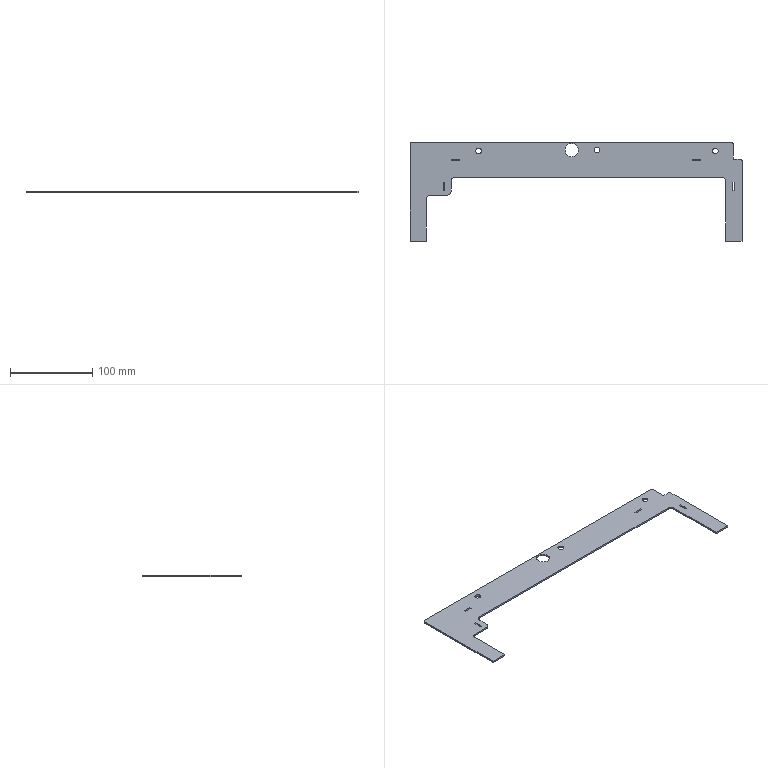Part | STEP file | xzz-001-2 | 1 solid | 45 faces | box 404 x 120 x 2 mm | volume 40299 mm3 | plane 30 | cylinder 15 | commonest cylinder face diameters 7 x6 10 x4 4 x3 16 x2
STEP:
#1=CARTESIAN_POINT('',(-138.,42.,-2.));
#2=VERTEX_POINT('',#1);
#3=CARTESIAN_POINT('',(-145.,42.,-2.));
#4=VERTEX_POINT('',#3);
#5=CARTESIAN_POINT('',(-141.5,42.,-2.));
#6=DIRECTION('',(0.,0.,-1.));
#7=DIRECTION('',(1.,0.,0.));
#8=AXIS2_PLACEMENT_3D('',#5,#6,#7);
#9=CIRCLE('',#8,3.5);
#10=EDGE_CURVE('',#2,#4,#9,.T.);
#11=ORIENTED_EDGE('',*,*,#10,.T.);
#12=CARTESIAN_POINT('',(-145.,42.,0.));
#13=VERTEX_POINT('',#12);
#14=CARTESIAN_POINT('',(-145.,42.,-2.));
#15=DIRECTION('',(0.,0.,1.));
#16=VECTOR('',#15,1000.);
#17=LINE('',#14,#16);
#18=EDGE_CURVE('',#4,#13,#17,.T.);
#19=ORIENTED_EDGE('',*,*,#18,.T.);
#20=CARTESIAN_POINT('',(-138.,42.,0.));
#21=VERTEX_POINT('',#20);
#22=CARTESIAN_POINT('',(-141.5,42.,0.));
#23=DIRECTION('',(0.,0.,-1.));
#24=DIRECTION('',(1.,0.,0.));
#25=AXIS2_PLACEMENT_3D('',#22,#23,#24);
#26=CIRCLE('',#25,3.5);
#27=EDGE_CURVE('',#21,#13,#26,.T.);
#28=ORIENTED_EDGE('',*,*,#27,.F.);
#29=CARTESIAN_POINT('',(-138.,42.,-2.));
#30=DIRECTION('',(0.,0.,1.));
#31=VECTOR('',#30,1000.);
#32=LINE('',#29,#31);
#33=EDGE_CURVE('',#2,#21,#32,.T.);
#34=ORIENTED_EDGE('',*,*,#33,.F.);
#35=EDGE_LOOP('',(#11,#19,#28,#34));
#36=FACE_OUTER_BOUND('',#35,.T.);
#37=CARTESIAN_POINT('',(-141.5,42.,-2.));
#38=DIRECTION('',(0.,0.,1.));
#39=DIRECTION('',(1.,0.,0.));
#40=AXIS2_PLACEMENT_3D('',#37,#38,#39);
#41=CYLINDRICAL_SURFACE('',#40,3.5);
#42=ADVANCED_FACE('',(#36),#41,.F.);
#43=CARTESIAN_POINT('',(6.,43.,-2.));
#44=VERTEX_POINT('',#43);
#45=CARTESIAN_POINT('',(-1.,43.,-2.));
#46=VERTEX_POINT('',#45);
#47=CARTESIAN_POINT('',(2.5,43.,-2.));
#48=DIRECTION('',(0.,0.,-1.));
#49=DIRECTION('',(1.,0.,0.));
#50=AXIS2_PLACEMENT_3D('',#47,#48,#49);
#51=CIRCLE('',#50,3.5);
#52=EDGE_CURVE('',#44,#46,#51,.T.);
#53=ORIENTED_EDGE('',*,*,#52,.T.);
#54=CARTESIAN_POINT('',(-1.,43.,0.));
#55=VERTEX_POINT('',#54);
#56=CARTESIAN_POINT('',(-1.,43.,-2.));
#57=DIRECTION('',(0.,0.,1.));
#58=VECTOR('',#57,1000.);
#59=LINE('',#56,#58);
#60=EDGE_CURVE('',#46,#55,#59,.T.);
#61=ORIENTED_EDGE('',*,*,#60,.T.);
#62=CARTESIAN_POINT('',(6.,43.,0.));
#63=VERTEX_POINT('',#62);
#64=CARTESIAN_POINT('',(2.5,43.,0.));
#65=DIRECTION('',(0.,0.,-1.));
#66=DIRECTION('',(1.,0.,0.));
#67=AXIS2_PLACEMENT_3D('',#64,#65,#66);
#68=CIRCLE('',#67,3.5);
#69=EDGE_CURVE('',#63,#55,#68,.T.);
#70=ORIENTED_EDGE('',*,*,#69,.F.);
#71=CARTESIAN_POINT('',(6.,43.,-2.));
#72=DIRECTION('',(0.,0.,1.));
#73=VECTOR('',#72,1000.);
#74=LINE('',#71,#73);
#75=EDGE_CURVE('',#44,#63,#74,.T.);
#76=ORIENTED_EDGE('',*,*,#75,.F.);
#77=EDGE_LOOP('',(#53,#61,#70,#76));
#78=FACE_OUTER_BOUND('',#77,.T.);
#79=CARTESIAN_POINT('',(2.5,43.,-2.));
#80=DIRECTION('',(0.,0.,1.));
#81=DIRECTION('',(1.,0.,0.));
#82=AXIS2_PLACEMENT_3D('',#79,#80,#81);
#83=CYLINDRICAL_SURFACE('',#82,3.5);
#84=ADVANCED_FACE('',(#78),#83,.F.);
#85=CARTESIAN_POINT('',(150.,42.,-2.));
#86=VERTEX_POINT('',#85);
#87=CARTESIAN_POINT('',(143.,42.,-2.));
#88=VERTEX_POINT('',#87);
#89=CARTESIAN_POINT('',(146.5,42.,-2.));
#90=DIRECTION('',(0.,0.,-1.));
#91=DIRECTION('',(1.,0.,0.));
#92=AXIS2_PLACEMENT_3D('',#89,#90,#91);
#93=CIRCLE('',#92,3.5);
#94=EDGE_CURVE('',#86,#88,#93,.T.);
#95=ORIENTED_EDGE('',*,*,#94,.T.);
#96=CARTESIAN_POINT('',(143.,42.,0.));
#97=VERTEX_POINT('',#96);
#98=CARTESIAN_POINT('',(143.,42.,-2.));
#99=DIRECTION('',(0.,0.,1.));
#100=VECTOR('',#99,1000.);
#101=LINE('',#98,#100);
#102=EDGE_CURVE('',#88,#97,#101,.T.);
#103=ORIENTED_EDGE('',*,*,#102,.T.);
#104=CARTESIAN_POINT('',(150.,42.,0.));
#105=VERTEX_POINT('',#104);
#106=CARTESIAN_POINT('',(146.5,42.,0.));
#107=DIRECTION('',(0.,0.,-1.));
#108=DIRECTION('',(1.,0.,0.));
#109=AXIS2_PLACEMENT_3D('',#106,#107,#108);
#110=CIRCLE('',#109,3.5);
#111=EDGE_CURVE('',#105,#97,#110,.T.);
#112=ORIENTED_EDGE('',*,*,#111,.F.);
#113=CARTESIAN_POINT('',(150.,42.,-2.));
#114=DIRECTION('',(0.,0.,1.));
#115=VECTOR('',#114,1000.);
#116=LINE('',#113,#115);
#117=EDGE_CURVE('',#86,#105,#116,.T.);
#118=ORIENTED_EDGE('',*,*,#117,.F.);
#119=EDGE_LOOP('',(#95,#103,#112,#118));
#120=FACE_OUTER_BOUND('',#119,.T.);
#121=CARTESIAN_POINT('',(146.5,42.,-2.));
#122=DIRECTION('',(0.,0.,1.));
#123=DIRECTION('',(1.,0.,0.));
#124=AXIS2_PLACEMENT_3D('',#121,#122,#123);
#125=CYLINDRICAL_SURFACE('',#124,3.5);
#126=ADVANCED_FACE('',(#120),#125,.F.);
#127=CARTESIAN_POINT('',(-20.25,43.,0.));
#128=VERTEX_POINT('',#127);
#129=CARTESIAN_POINT('',(-36.25,43.,0.));
#130=VERTEX_POINT('',#129);
#131=CARTESIAN_POINT('',(-28.25,43.,0.));
#132=DIRECTION('',(0.,0.,-1.));
#133=DIRECTION('',(-1.,0.,0.));
#134=AXIS2_PLACEMENT_3D('',#131,#132,#133);
#135=CIRCLE('',#134,8.);
#136=EDGE_CURVE('',#128,#130,#135,.T.);
#137=ORIENTED_EDGE('',*,*,#136,.F.);
#138=CARTESIAN_POINT('',(-20.25,43.,-2.));
#139=VERTEX_POINT('',#138);
#140=CARTESIAN_POINT('',(-20.25,43.,8.));
#141=DIRECTION('',(0.,0.,-1.));
#142=VECTOR('',#141,1000.);
#143=LINE('',#140,#142);
#144=EDGE_CURVE('',#128,#139,#143,.T.);
#145=ORIENTED_EDGE('',*,*,#144,.T.);
#146=CARTESIAN_POINT('',(-36.25,43.,-2.));
#147=VERTEX_POINT('',#146);
#148=CARTESIAN_POINT('',(-28.25,43.,-2.));
#149=DIRECTION('',(0.,0.,-1.));
#150=DIRECTION('',(-1.,0.,0.));
#151=AXIS2_PLACEMENT_3D('',#148,#149,#150);
#152=CIRCLE('',#151,8.);
#153=EDGE_CURVE('',#139,#147,#152,.T.);
#154=ORIENTED_EDGE('',*,*,#153,.T.);
#155=CARTESIAN_POINT('',(-36.25,43.,8.));
#156=DIRECTION('',(0.,0.,-1.));
#157=VECTOR('',#156,1000.);
#158=LINE('',#155,#157);
#159=EDGE_CURVE('',#130,#147,#158,.T.);
#160=ORIENTED_EDGE('',*,*,#159,.F.);
#161=EDGE_LOOP('',(#137,#145,#154,#160));
#162=FACE_OUTER_BOUND('',#161,.T.);
#163=CARTESIAN_POINT('',(-28.25,43.,8.));
#164=DIRECTION('',(0.,0.,-1.));
#165=DIRECTION('',(-1.,0.,0.));
#166=AXIS2_PLACEMENT_3D('',#163,#164,#165);
#167=CYLINDRICAL_SURFACE('',#166,8.);
#168=ADVANCED_FACE('',(#162),#167,.F.);
#169=ORIENTED_EDGE('',*,*,#10,.F.);
#170=CARTESIAN_POINT('',(-141.5,42.,-2.));
#171=DIRECTION('',(0.,0.,-1.));
#172=DIRECTION('',(1.,0.,0.));
#173=AXIS2_PLACEMENT_3D('',#170,#171,#172);
#174=CIRCLE('',#173,3.5);
#175=EDGE_CURVE('',#4,#2,#174,.T.);
#176=ORIENTED_EDGE('',*,*,#175,.F.);
#177=EDGE_LOOP('',(#169,#176));
#178=FACE_BOUND('',#177,.T.);
#179=ORIENTED_EDGE('',*,*,#52,.F.);
#180=CARTESIAN_POINT('',(2.5,43.,-2.));
#181=DIRECTION('',(0.,0.,-1.));
#182=DIRECTION('',(1.,0.,0.));
#183=AXIS2_PLACEMENT_3D('',#180,#181,#182);
#184=CIRCLE('',#183,3.5);
#185=EDGE_CURVE('',#46,#44,#184,.T.);
#186=ORIENTED_EDGE('',*,*,#185,.F.);
#187=EDGE_LOOP('',(#179,#186));
#188=FACE_BOUND('',#187,.T.);
#189=ORIENTED_EDGE('',*,*,#94,.F.);
#190=CARTESIAN_POINT('',(146.5,42.,-2.));
#191=DIRECTION('',(0.,0.,-1.));
#192=DIRECTION('',(1.,0.,0.));
#193=AXIS2_PLACEMENT_3D('',#190,#191,#192);
#194=CIRCLE('',#193,3.5);
#195=EDGE_CURVE('',#88,#86,#194,.T.);
#196=ORIENTED_EDGE('',*,*,#195,.F.);
#197=EDGE_LOOP('',(#189,#196));
#198=FACE_BOUND('',#197,.T.);
#199=CARTESIAN_POINT('',(-175.,30.,-2.));
#200=VERTEX_POINT('',#199);
#201=CARTESIAN_POINT('',(-175.,32.,-2.));
#202=VERTEX_POINT('',#201);
#203=CARTESIAN_POINT('',(-175.,0.,-2.));
#204=DIRECTION('',(0.,1.,0.));
#205=VECTOR('',#204,1000.);
#206=LINE('',#203,#205);
#207=EDGE_CURVE('',#200,#202,#206,.T.);
#208=ORIENTED_EDGE('',*,*,#207,.F.);
#209=CARTESIAN_POINT('',(-165.,30.,-2.));
#210=VERTEX_POINT('',#209);
#211=CARTESIAN_POINT('',(0.,30.,-2.));
#212=DIRECTION('',(-1.,0.,0.));
#213=VECTOR('',#212,1000.);
#214=LINE('',#211,#213);
#215=EDGE_CURVE('',#210,#200,#214,.T.);
#216=ORIENTED_EDGE('',*,*,#215,.F.);
#217=CARTESIAN_POINT('',(-165.,32.,-2.));
#218=VERTEX_POINT('',#217);
#219=CARTESIAN_POINT('',(-165.,0.,-2.));
#220=DIRECTION('',(0.,-1.,0.));
#221=VECTOR('',#220,1000.);
#222=LINE('',#219,#221);
#223=EDGE_CURVE('',#218,#210,#222,.T.);
#224=ORIENTED_EDGE('',*,*,#223,.F.);
#225=CARTESIAN_POINT('',(0.,32.,-2.));
#226=DIRECTION('',(1.,0.,0.));
#227=VECTOR('',#226,1000.);
#228=LINE('',#225,#227);
#229=EDGE_CURVE('',#202,#218,#228,.T.);
#230=ORIENTED_EDGE('',*,*,#229,.F.);
#231=EDGE_LOOP('',(#208,#216,#224,#230));
#232=FACE_BOUND('',#231,.T.);
#233=CARTESIAN_POINT('',(119.,30.,-2.));
#234=VERTEX_POINT('',#233);
#235=CARTESIAN_POINT('',(119.,32.,-2.));
#236=VERTEX_POINT('',#235);
#237=CARTESIAN_POINT('',(119.,0.,-2.));
#238=DIRECTION('',(0.,1.,0.));
#239=VECTOR('',#238,1000.);
#240=LINE('',#237,#239);
#241=EDGE_CURVE('',#234,#236,#240,.T.);
#242=ORIENTED_EDGE('',*,*,#241,.F.);
#243=CARTESIAN_POINT('',(129.,30.,-2.));
#244=VERTEX_POINT('',#243);
#245=CARTESIAN_POINT('',(0.,30.,-2.));
#246=DIRECTION('',(-1.,0.,0.));
#247=VECTOR('',#246,1000.);
#248=LINE('',#245,#247);
#249=EDGE_CURVE('',#244,#234,#248,.T.);
#250=ORIENTED_EDGE('',*,*,#249,.F.);
#251=CARTESIAN_POINT('',(129.,32.,-2.));
#252=VERTEX_POINT('',#251);
#253=CARTESIAN_POINT('',(129.,0.,-2.));
#254=DIRECTION('',(0.,-1.,0.));
#255=VECTOR('',#254,1000.);
#256=LINE('',#253,#255);
#257=EDGE_CURVE('',#252,#244,#256,.T.);
#258=ORIENTED_EDGE('',*,*,#257,.F.);
#259=CARTESIAN_POINT('',(0.,32.,-2.));
#260=DIRECTION('',(1.,0.,0.));
#261=VECTOR('',#260,1000.);
#262=LINE('',#259,#261);
#263=EDGE_CURVE('',#236,#252,#262,.T.);
#264=ORIENTED_EDGE('',*,*,#263,.F.);
#265=EDGE_LOOP('',(#242,#250,#258,#264));
#266=FACE_BOUND('',#265,.T.);
#267=CARTESIAN_POINT('',(-223.,52.,-2.));
#268=VERTEX_POINT('',#267);
#269=CARTESIAN_POINT('',(-225.,50.,-2.));
#270=VERTEX_POINT('',#269);
#271=CARTESIAN_POINT('',(-223.,50.,-2.));
#272=DIRECTION('',(0.,0.,1.));
#273=DIRECTION('',(1.,0.,0.));
#274=AXIS2_PLACEMENT_3D('',#271,#272,#273);
#275=CIRCLE('',#274,2.);
#276=EDGE_CURVE('',#268,#270,#275,.T.);
#277=ORIENTED_EDGE('',*,*,#276,.F.);
#278=CARTESIAN_POINT('',(166.5,52.,-2.));
#279=VERTEX_POINT('',#278);
#280=CARTESIAN_POINT('',(0.,52.,-2.));
#281=DIRECTION('',(-1.,0.,0.));
#282=VECTOR('',#281,1000.);
#283=LINE('',#280,#282);
#284=EDGE_CURVE('',#279,#268,#283,.T.);
#285=ORIENTED_EDGE('',*,*,#284,.F.);
#286=CARTESIAN_POINT('',(168.5,50.,-2.));
#287=VERTEX_POINT('',#286);
#288=CARTESIAN_POINT('',(166.5,50.,-2.));
#289=DIRECTION('',(0.,0.,1.));
#290=DIRECTION('',(1.,0.,0.));
#291=AXIS2_PLACEMENT_3D('',#288,#289,#290);
#292=CIRCLE('',#291,2.);
#293=EDGE_CURVE('',#287,#279,#292,.T.);
#294=ORIENTED_EDGE('',*,*,#293,.F.);
#295=CARTESIAN_POINT('',(168.5,32.,-2.));
#296=VERTEX_POINT('',#295);
#297=CARTESIAN_POINT('',(168.5,0.,-2.));
#298=DIRECTION('',(0.,1.,0.));
#299=VECTOR('',#298,1000.);
#300=LINE('',#297,#299);
#301=EDGE_CURVE('',#296,#287,#300,.T.);
#302=ORIENTED_EDGE('',*,*,#301,.F.);
#303=CARTESIAN_POINT('',(177.,32.,-2.));
#304=VERTEX_POINT('',#303);
#305=CARTESIAN_POINT('',(0.,32.,-2.));
#306=DIRECTION('',(-1.,0.,0.));
#307=VECTOR('',#306,1000.);
#308=LINE('',#305,#307);
#309=EDGE_CURVE('',#304,#296,#308,.T.);
#310=ORIENTED_EDGE('',*,*,#309,.F.);
#311=CARTESIAN_POINT('',(179.,30.,-2.));
#312=VERTEX_POINT('',#311);
#313=CARTESIAN_POINT('',(177.,30.,-2.));
#314=DIRECTION('',(0.,0.,1.));
#315=DIRECTION('',(1.,0.,0.));
#316=AXIS2_PLACEMENT_3D('',#313,#314,#315);
#317=CIRCLE('',#316,2.);
#318=EDGE_CURVE('',#312,#304,#317,.T.);
#319=ORIENTED_EDGE('',*,*,#318,.F.);
#320=CARTESIAN_POINT('',(179.,-68.,-2.));
#321=VERTEX_POINT('',#320);
#322=CARTESIAN_POINT('',(179.,0.,-2.));
#323=DIRECTION('',(0.,1.,0.));
#324=VECTOR('',#323,1000.);
#325=LINE('',#322,#324);
#326=EDGE_CURVE('',#321,#312,#325,.T.);
#327=ORIENTED_EDGE('',*,*,#326,.F.);
#328=CARTESIAN_POINT('',(159.,-68.,-2.));
#329=VERTEX_POINT('',#328);
#330=CARTESIAN_POINT('',(0.,-68.,-2.));
#331=DIRECTION('',(1.,0.,0.));
#332=VECTOR('',#331,1000.);
#333=LINE('',#330,#332);
#334=EDGE_CURVE('',#329,#321,#333,.T.);
#335=ORIENTED_EDGE('',*,*,#334,.F.);
#336=CARTESIAN_POINT('',(159.,5.,-2.));
#337=VERTEX_POINT('',#336);
#338=CARTESIAN_POINT('',(159.,0.,-2.));
#339=DIRECTION('',(0.,-1.,0.));
#340=VECTOR('',#339,1000.);
#341=LINE('',#338,#340);
#342=EDGE_CURVE('',#337,#329,#341,.T.);
#343=ORIENTED_EDGE('',*,*,#342,.F.);
#344=CARTESIAN_POINT('',(154.,10.,-2.));
#345=VERTEX_POINT('',#344);
#346=CARTESIAN_POINT('',(154.,5.,-2.));
#347=DIRECTION('',(0.,0.,-1.));
#348=DIRECTION('',(-1.,0.,0.));
#349=AXIS2_PLACEMENT_3D('',#346,#347,#348);
#350=CIRCLE('',#349,5.);
#351=EDGE_CURVE('',#345,#337,#350,.T.);
#352=ORIENTED_EDGE('',*,*,#351,.F.);
#353=CARTESIAN_POINT('',(-170.,10.,-2.));
#354=VERTEX_POINT('',#353);
#355=CARTESIAN_POINT('',(0.,10.,-2.));
#356=DIRECTION('',(1.,0.,0.));
#357=VECTOR('',#356,1000.);
#358=LINE('',#355,#357);
#359=EDGE_CURVE('',#354,#345,#358,.T.);
#360=ORIENTED_EDGE('',*,*,#359,.F.);
#361=CARTESIAN_POINT('',(-175.,5.,-2.));
#362=VERTEX_POINT('',#361);
#363=CARTESIAN_POINT('',(-170.,5.,-2.));
#364=DIRECTION('',(0.,0.,-1.));
#365=DIRECTION('',(1.,0.,0.));
#366=AXIS2_PLACEMENT_3D('',#363,#364,#365);
#367=CIRCLE('',#366,5.);
#368=EDGE_CURVE('',#362,#354,#367,.T.);
#369=ORIENTED_EDGE('',*,*,#368,.F.);
#370=CARTESIAN_POINT('',(-175.,-7.,-2.));
#371=VERTEX_POINT('',#370);
#372=CARTESIAN_POINT('',(-175.,0.,-2.));
#373=DIRECTION('',(0.,1.,0.));
#374=VECTOR('',#373,1000.);
#375=LINE('',#372,#374);
#376=EDGE_CURVE('',#371,#362,#375,.T.);
#377=ORIENTED_EDGE('',*,*,#376,.F.);
#378=CARTESIAN_POINT('',(-180.,-12.,-2.));
#379=VERTEX_POINT('',#378);
#380=CARTESIAN_POINT('',(-180.,-7.,-2.));
#381=DIRECTION('',(0.,0.,1.));
#382=DIRECTION('',(-1.,0.,0.));
#383=AXIS2_PLACEMENT_3D('',#380,#381,#382);
#384=CIRCLE('',#383,5.);
#385=EDGE_CURVE('',#379,#371,#384,.T.);
#386=ORIENTED_EDGE('',*,*,#385,.F.);
#387=CARTESIAN_POINT('',(-200.,-12.,-2.));
#388=VERTEX_POINT('',#387);
#389=CARTESIAN_POINT('',(0.,-12.,-2.));
#390=DIRECTION('',(1.,0.,0.));
#391=VECTOR('',#390,1000.);
#392=LINE('',#389,#391);
#393=EDGE_CURVE('',#388,#379,#392,.T.);
#394=ORIENTED_EDGE('',*,*,#393,.F.);
#395=CARTESIAN_POINT('',(-205.,-17.,-2.));
#396=VERTEX_POINT('',#395);
#397=CARTESIAN_POINT('',(-200.,-17.,-2.));
#398=DIRECTION('',(0.,0.,-1.));
#399=DIRECTION('',(1.,0.,0.));
#400=AXIS2_PLACEMENT_3D('',#397,#398,#399);
#401=CIRCLE('',#400,5.);
#402=EDGE_CURVE('',#396,#388,#401,.T.);
#403=ORIENTED_EDGE('',*,*,#402,.F.);
#404=CARTESIAN_POINT('',(-205.,-68.,-2.));
#405=VERTEX_POINT('',#404);
#406=CARTESIAN_POINT('',(-205.,0.,-2.));
#407=DIRECTION('',(0.,1.,0.));
#408=VECTOR('',#407,1000.);
#409=LINE('',#406,#408);
#410=EDGE_CURVE('',#405,#396,#409,.T.);
#411=ORIENTED_EDGE('',*,*,#410,.F.);
#412=CARTESIAN_POINT('',(-225.,-68.,-2.));
#413=VERTEX_POINT('',#412);
#414=CARTESIAN_POINT('',(0.,-68.,-2.));
#415=DIRECTION('',(1.,0.,0.));
#416=VECTOR('',#415,1000.);
#417=LINE('',#414,#416);
#418=EDGE_CURVE('',#413,#405,#417,.T.);
#419=ORIENTED_EDGE('',*,*,#418,.F.);
#420=CARTESIAN_POINT('',(-225.,0.,-2.));
#421=DIRECTION('',(0.,-1.,0.));
#422=VECTOR('',#421,1000.);
#423=LINE('',#420,#422);
#424=EDGE_CURVE('',#270,#413,#423,.T.);
#425=ORIENTED_EDGE('',*,*,#424,.F.);
#426=EDGE_LOOP('',(#277,#285,#294,#302,#310,#319,#327,#335,#343,#352,#360,#369,#377,#386,#394,#403,#411,#419,#425));
#427=FACE_OUTER_BOUND('',#426,.T.);
#428=CARTESIAN_POINT('',(169.5,4.,-2.));
#429=VERTEX_POINT('',#428);
#430=CARTESIAN_POINT('',(169.5,-6.,-2.));
#431=VERTEX_POINT('',#430);
#432=CARTESIAN_POINT('',(169.5,0.,-2.));
#433=DIRECTION('',(0.,-1.,0.));
#434=VECTOR('',#433,1000.);
#435=LINE('',#432,#434);
#436=EDGE_CURVE('',#429,#431,#435,.T.);
#437=ORIENTED_EDGE('',*,*,#436,.F.);
#438=CARTESIAN_POINT('',(167.5,4.,-2.));
#439=VERTEX_POINT('',#438);
#440=CARTESIAN_POINT('',(0.,4.,-2.));
#441=DIRECTION('',(1.,0.,0.));
#442=VECTOR('',#441,1000.);
#443=LINE('',#440,#442);
#444=EDGE_CURVE('',#439,#429,#443,.T.);
#445=ORIENTED_EDGE('',*,*,#444,.F.);
#446=CARTESIAN_POINT('',(167.5,-6.,-2.));
#447=VERTEX_POINT('',#446);
#448=CARTESIAN_POINT('',(167.5,0.,-2.));
#449=DIRECTION('',(0.,1.,0.));
#450=VECTOR('',#449,1000.);
#451=LINE('',#448,#450);
#452=EDGE_CURVE('',#447,#439,#451,.T.);
#453=ORIENTED_EDGE('',*,*,#452,.F.);
#454=CARTESIAN_POINT('',(0.,-6.,-2.));
#455=DIRECTION('',(-1.,0.,0.));
#456=VECTOR('',#455,1000.);
#457=LINE('',#454,#456);
#458=EDGE_CURVE('',#431,#447,#457,.T.);
#459=ORIENTED_EDGE('',*,*,#458,.F.);
#460=EDGE_LOOP('',(#437,#445,#453,#459));
#461=FACE_BOUND('',#460,.T.);
#462=CARTESIAN_POINT('',(-182.5,4.,-2.));
#463=VERTEX_POINT('',#462);
#464=CARTESIAN_POINT('',(-182.5,-6.,-2.));
#465=VERTEX_POINT('',#464);
#466=CARTESIAN_POINT('',(-182.5,0.,-2.));
#467=DIRECTION('',(0.,-1.,0.));
#468=VECTOR('',#467,1000.);
#469=LINE('',#466,#468);
#470=EDGE_CURVE('',#463,#465,#469,.T.);
#471=ORIENTED_EDGE('',*,*,#470,.F.);
#472=CARTESIAN_POINT('',(-184.5,4.,-2.));
#473=VERTEX_POINT('',#472);
#474=CARTESIAN_POINT('',(0.,4.,-2.));
#475=DIRECTION('',(1.,0.,0.));
#476=VECTOR('',#475,1000.);
#477=LINE('',#474,#476);
#478=EDGE_CURVE('',#473,#463,#477,.T.);
#479=ORIENTED_EDGE('',*,*,#478,.F.);
#480=CARTESIAN_POINT('',(-184.5,-6.,-2.));
#481=VERTEX_POINT('',#480);
#482=CARTESIAN_POINT('',(-184.5,0.,-2.));
#483=DIRECTION('',(0.,1.,0.));
#484=VECTOR('',#483,1000.);
#485=LINE('',#482,#484);
#486=EDGE_CURVE('',#481,#473,#485,.T.);
#487=ORIENTED_EDGE('',*,*,#486,.F.);
#488=CARTESIAN_POINT('',(0.,-6.,-2.));
#489=DIRECTION('',(-1.,0.,0.));
#490=VECTOR('',#489,1000.);
#491=LINE('',#488,#490);
#492=EDGE_CURVE('',#465,#481,#491,.T.);
#493=ORIENTED_EDGE('',*,*,#492,.F.);
#494=EDGE_LOOP('',(#471,#479,#487,#493));
#495=FACE_BOUND('',#494,.T.);
#496=CARTESIAN_POINT('',(-28.25,43.,-2.));
#497=DIRECTION('',(0.,0.,-1.));
#498=DIRECTION('',(-1.,0.,0.));
#499=AXIS2_PLACEMENT_3D('',#496,#497,#498);
#500=CIRCLE('',#499,8.);
#501=EDGE_CURVE('',#147,#139,#500,.T.);
#502=ORIENTED_EDGE('',*,*,#501,.F.);
#503=ORIENTED_EDGE('',*,*,#153,.F.);
#504=EDGE_LOOP('',(#502,#503));
#505=FACE_BOUND('',#504,.T.);
#506=CARTESIAN_POINT('',(0.,0.,-2.));
#507=DIRECTION('',(0.,0.,1.));
#508=DIRECTION('',(1.,0.,0.));
#509=AXIS2_PLACEMENT_3D('',#506,#507,#508);
#510=PLANE('',#509);
#511=ADVANCED_FACE('',(#178,#188,#198,#232,#266,#427,#461,#495,#505),#510,.F.);
#512=ORIENTED_EDGE('',*,*,#18,.F.);
#513=ORIENTED_EDGE('',*,*,#175,.T.);
#514=ORIENTED_EDGE('',*,*,#33,.T.);
#515=CARTESIAN_POINT('',(-141.5,42.,0.));
#516=DIRECTION('',(0.,0.,-1.));
#517=DIRECTION('',(1.,0.,0.));
#518=AXIS2_PLACEMENT_3D('',#515,#516,#517);
#519=CIRCLE('',#518,3.5);
#520=EDGE_CURVE('',#13,#21,#519,.T.);
#521=ORIENTED_EDGE('',*,*,#520,.F.);
#522=EDGE_LOOP('',(#512,#513,#514,#521));
#523=FACE_OUTER_BOUND('',#522,.T.);
#524=CARTESIAN_POINT('',(-141.5,42.,-2.));
#525=DIRECTION('',(0.,0.,1.));
#526=DIRECTION('',(1.,0.,0.));
#527=AXIS2_PLACEMENT_3D('',#524,#525,#526);
#528=CYLINDRICAL_SURFACE('',#527,3.5);
#529=ADVANCED_FACE('',(#523),#528,.F.);
#530=ORIENTED_EDGE('',*,*,#60,.F.);
#531=ORIENTED_EDGE('',*,*,#185,.T.);
#532=ORIENTED_EDGE('',*,*,#75,.T.);
#533=CARTESIAN_POINT('',(2.5,43.,0.));
#534=DIRECTION('',(0.,0.,-1.));
#535=DIRECTION('',(1.,0.,0.));
#536=AXIS2_PLACEMENT_3D('',#533,#534,#535);
#537=CIRCLE('',#536,3.5);
#538=EDGE_CURVE('',#55,#63,#537,.T.);
#539=ORIENTED_EDGE('',*,*,#538,.F.);
#540=EDGE_LOOP('',(#530,#531,#532,#539));
#541=FACE_OUTER_BOUND('',#540,.T.);
#542=CARTESIAN_POINT('',(2.5,43.,-2.));
#543=DIRECTION('',(0.,0.,1.));
#544=DIRECTION('',(1.,0.,0.));
#545=AXIS2_PLACEMENT_3D('',#542,#543,#544);
#546=CYLINDRICAL_SURFACE('',#545,3.5);
#547=ADVANCED_FACE('',(#541),#546,.F.);
#548=ORIENTED_EDGE('',*,*,#102,.F.);
#549=ORIENTED_EDGE('',*,*,#195,.T.);
#550=ORIENTED_EDGE('',*,*,#117,.T.);
#551=CARTESIAN_POINT('',(146.5,42.,0.));
#552=DIRECTION('',(0.,0.,-1.));
#553=DIRECTION('',(1.,0.,0.));
#554=AXIS2_PLACEMENT_3D('',#551,#552,#553);
#555=CIRCLE('',#554,3.5);
#556=EDGE_CURVE('',#97,#105,#555,.T.);
#557=ORIENTED_EDGE('',*,*,#556,.F.);
#558=EDGE_LOOP('',(#548,#549,#550,#557));
#559=FACE_OUTER_BOUND('',#558,.T.);
#560=CARTESIAN_POINT('',(146.5,42.,-2.));
#561=DIRECTION('',(0.,0.,1.));
#562=DIRECTION('',(1.,0.,0.));
#563=AXIS2_PLACEMENT_3D('',#560,#561,#562);
#564=CYLINDRICAL_SURFACE('',#563,3.5);
#565=ADVANCED_FACE('',(#559),#564,.F.);
#566=CARTESIAN_POINT('',(-175.,32.,0.));
#567=VERTEX_POINT('',#566);
#568=CARTESIAN_POINT('',(-165.,32.,0.));
#569=VERTEX_POINT('',#568);
#570=CARTESIAN_POINT('',(-175.,32.,0.));
#571=DIRECTION('',(1.,0.,0.));
#572=VECTOR('',#571,1000.);
#573=LINE('',#570,#572);
#574=EDGE_CURVE('',#567,#569,#573,.T.);
#575=ORIENTED_EDGE('',*,*,#574,.F.);
#576=CARTESIAN_POINT('',(-175.,32.,-10.));
#577=DIRECTION('',(0.,0.,1.));
#578=VECTOR('',#577,1000.);
#579=LINE('',#576,#578);
#580=EDGE_CURVE('',#202,#567,#579,.T.);
#581=ORIENTED_EDGE('',*,*,#580,.F.);
#582=ORIENTED_EDGE('',*,*,#229,.T.);
#583=CARTESIAN_POINT('',(-165.,32.,-10.));
#584=DIRECTION('',(0.,0.,-1.));
#585=VECTOR('',#584,1000.);
#586=LINE('',#583,#585);
#587=EDGE_CURVE('',#569,#218,#586,.T.);
#588=ORIENTED_EDGE('',*,*,#587,.F.);
#589=EDGE_LOOP('',(#575,#581,#582,#588));
#590=FACE_OUTER_BOUND('',#589,.T.);
#591=CARTESIAN_POINT('',(-175.,32.,-10.));
#592=DIRECTION('',(0.,1.,0.));
#593=DIRECTION('',(0.,0.,1.));
#594=AXIS2_PLACEMENT_3D('',#591,#592,#593);
#595=PLANE('',#594);
#596=ADVANCED_FACE('',(#590),#595,.F.);
#597=CARTESIAN_POINT('',(-175.,30.,0.));
#598=VERTEX_POINT('',#597);
#599=CARTESIAN_POINT('',(-175.,32.,0.));
#600=DIRECTION('',(0.,1.,0.));
#601=VECTOR('',#600,1000.);
#602=LINE('',#599,#601);
#603=EDGE_CURVE('',#598,#567,#602,.T.);
#604=ORIENTED_EDGE('',*,*,#603,.F.);
#605=CARTESIAN_POINT('',(-175.,30.,-10.));
#606=DIRECTION('',(0.,0.,1.));
#607=VECTOR('',#606,1000.);
#608=LINE('',#605,#607);
#609=EDGE_CURVE('',#200,#598,#608,.T.);
#610=ORIENTED_EDGE('',*,*,#609,.F.);
#611=ORIENTED_EDGE('',*,*,#207,.T.);
#612=ORIENTED_EDGE('',*,*,#580,.T.);
#613=EDGE_LOOP('',(#604,#610,#611,#612));
#614=FACE_OUTER_BOUND('',#613,.T.);
#615=CARTESIAN_POINT('',(-175.,32.,-10.));
#616=DIRECTION('',(-1.,0.,0.));
#617=DIRECTION('',(0.,0.,1.));
#618=AXIS2_PLACEMENT_3D('',#615,#616,#617);
#619=PLANE('',#618);
#620=ADVANCED_FACE('',(#614),#619,.F.);
#621=CARTESIAN_POINT('',(-165.,30.,0.));
#622=VERTEX_POINT('',#621);
#623=CARTESIAN_POINT('',(-175.,30.,0.));
#624=DIRECTION('',(-1.,0.,0.));
#625=VECTOR('',#624,1000.);
#626=LINE('',#623,#625);
#627=EDGE_CURVE('',#622,#598,#626,.T.);
#628=ORIENTED_EDGE('',*,*,#627,.F.);
#629=CARTESIAN_POINT('',(-165.,30.,-10.));
#630=DIRECTION('',(0.,0.,1.));
#631=VECTOR('',#630,1000.);
#632=LINE('',#629,#631);
#633=EDGE_CURVE('',#210,#622,#632,.T.);
#634=ORIENTED_EDGE('',*,*,#633,.F.);
#635=ORIENTED_EDGE('',*,*,#215,.T.);
#636=ORIENTED_EDGE('',*,*,#609,.T.);
#637=EDGE_LOOP('',(#628,#634,#635,#636));
#638=FACE_OUTER_BOUND('',#637,.T.);
#639=CARTESIAN_POINT('',(-175.,30.,-10.));
#640=DIRECTION('',(0.,-1.,0.));
#641=DIRECTION('',(0.,0.,-1.));
#642=AXIS2_PLACEMENT_3D('',#639,#640,#641);
#643=PLANE('',#642);
#644=ADVANCED_FACE('',(#638),#643,.F.);
#645=CARTESIAN_POINT('',(-165.,32.,0.));
#646=DIRECTION('',(0.,-1.,0.));
#647=VECTOR('',#646,1000.);
#648=LINE('',#645,#647);
#649=EDGE_CURVE('',#569,#622,#648,.T.);
#650=ORIENTED_EDGE('',*,*,#649,.F.);
#651=ORIENTED_EDGE('',*,*,#587,.T.);
#652=ORIENTED_EDGE('',*,*,#223,.T.);
#653=ORIENTED_EDGE('',*,*,#633,.T.);
#654=EDGE_LOOP('',(#650,#651,#652,#653));
#655=FACE_OUTER_BOUND('',#654,.T.);
#656=CARTESIAN_POINT('',(-165.,32.,-10.));
#657=DIRECTION('',(1.,0.,0.));
#658=DIRECTION('',(0.,0.,-1.));
#659=AXIS2_PLACEMENT_3D('',#656,#657,#658);
#660=PLANE('',#659);
#661=ADVANCED_FACE('',(#655),#660,.F.);
#662=CARTESIAN_POINT('',(119.,32.,0.));
#663=VERTEX_POINT('',#662);
#664=CARTESIAN_POINT('',(129.,32.,0.));
#665=VERTEX_POINT('',#664);
#666=CARTESIAN_POINT('',(119.,32.,0.));
#667=DIRECTION('',(1.,0.,0.));
#668=VECTOR('',#667,1000.);
#669=LINE('',#666,#668);
#670=EDGE_CURVE('',#663,#665,#669,.T.);
#671=ORIENTED_EDGE('',*,*,#670,.F.);
#672=CARTESIAN_POINT('',(119.,32.,-10.));
#673=DIRECTION('',(0.,0.,1.));
#674=VECTOR('',#673,1000.);
#675=LINE('',#672,#674);
#676=EDGE_CURVE('',#236,#663,#675,.T.);
#677=ORIENTED_EDGE('',*,*,#676,.F.);
#678=ORIENTED_EDGE('',*,*,#263,.T.);
#679=CARTESIAN_POINT('',(129.,32.,-10.));
#680=DIRECTION('',(0.,0.,-1.));
#681=VECTOR('',#680,1000.);
#682=LINE('',#679,#681);
#683=EDGE_CURVE('',#665,#252,#682,.T.);
#684=ORIENTED_EDGE('',*,*,#683,.F.);
#685=EDGE_LOOP('',(#671,#677,#678,#684));
#686=FACE_OUTER_BOUND('',#685,.T.);
#687=CARTESIAN_POINT('',(119.,32.,-10.));
#688=DIRECTION('',(0.,1.,0.));
#689=DIRECTION('',(0.,0.,1.));
#690=AXIS2_PLACEMENT_3D('',#687,#688,#689);
#691=PLANE('',#690);
#692=ADVANCED_FACE('',(#686),#691,.F.);
#693=CARTESIAN_POINT('',(119.,30.,0.));
#694=VERTEX_POINT('',#693);
#695=CARTESIAN_POINT('',(119.,32.,0.));
#696=DIRECTION('',(0.,1.,0.));
#697=VECTOR('',#696,1000.);
#698=LINE('',#695,#697);
#699=EDGE_CURVE('',#694,#663,#698,.T.);
#700=ORIENTED_EDGE('',*,*,#699,.F.);
#701=CARTESIAN_POINT('',(119.,30.,-10.));
#702=DIRECTION('',(0.,0.,1.));
#703=VECTOR('',#702,1000.);
#704=LINE('',#701,#703);
#705=EDGE_CURVE('',#234,#694,#704,.T.);
#706=ORIENTED_EDGE('',*,*,#705,.F.);
#707=ORIENTED_EDGE('',*,*,#241,.T.);
#708=ORIENTED_EDGE('',*,*,#676,.T.);
#709=EDGE_LOOP('',(#700,#706,#707,#708));
#710=FACE_OUTER_BOUND('',#709,.T.);
#711=CARTESIAN_POINT('',(119.,32.,-10.));
#712=DIRECTION('',(-1.,0.,0.));
#713=DIRECTION('',(0.,0.,1.));
#714=AXIS2_PLACEMENT_3D('',#711,#712,#713);
#715=PLANE('',#714);
#716=ADVANCED_FACE('',(#710),#715,.F.);
#717=CARTESIAN_POINT('',(129.,30.,0.));
#718=VERTEX_POINT('',#717);
#719=CARTESIAN_POINT('',(119.,30.,0.));
#720=DIRECTION('',(-1.,0.,0.));
#721=VECTOR('',#720,1000.);
#722=LINE('',#719,#721);
#723=EDGE_CURVE('',#718,#694,#722,.T.);
#724=ORIENTED_EDGE('',*,*,#723,.F.);
#725=CARTESIAN_POINT('',(129.,30.,-10.));
#726=DIRECTION('',(0.,0.,1.));
#727=VECTOR('',#726,1000.);
#728=LINE('',#725,#727);
#729=EDGE_CURVE('',#244,#718,#728,.T.);
#730=ORIENTED_EDGE('',*,*,#729,.F.);
#731=ORIENTED_EDGE('',*,*,#249,.T.);
#732=ORIENTED_EDGE('',*,*,#705,.T.);
#733=EDGE_LOOP('',(#724,#730,#731,#732));
#734=FACE_OUTER_BOUND('',#733,.T.);
#735=CARTESIAN_POINT('',(119.,30.,-10.));
#736=DIRECTION('',(0.,-1.,0.));
#737=DIRECTION('',(0.,0.,-1.));
#738=AXIS2_PLACEMENT_3D('',#735,#736,#737);
#739=PLANE('',#738);
#740=ADVANCED_FACE('',(#734),#739,.F.);
#741=CARTESIAN_POINT('',(129.,32.,0.));
#742=DIRECTION('',(0.,-1.,0.));
#743=VECTOR('',#742,1000.);
#744=LINE('',#741,#743);
#745=EDGE_CURVE('',#665,#718,#744,.T.);
#746=ORIENTED_EDGE('',*,*,#745,.F.);
#747=ORIENTED_EDGE('',*,*,#683,.T.);
#748=ORIENTED_EDGE('',*,*,#257,.T.);
#749=ORIENTED_EDGE('',*,*,#729,.T.);
#750=EDGE_LOOP('',(#746,#747,#748,#749));
#751=FACE_OUTER_BOUND('',#750,.T.);
#752=CARTESIAN_POINT('',(129.,32.,-10.));
#753=DIRECTION('',(1.,0.,0.));
#754=DIRECTION('',(0.,0.,-1.));
#755=AXIS2_PLACEMENT_3D('',#752,#753,#754);
#756=PLANE('',#755);
#757=ADVANCED_FACE('',(#751),#756,.F.);
#758=ORIENTED_EDGE('',*,*,#424,.T.);
#759=CARTESIAN_POINT('',(-225.,-68.,0.));
#760=VERTEX_POINT('',#759);
#761=CARTESIAN_POINT('',(-225.,-68.,-2.));
#762=DIRECTION('',(0.,0.,1.));
#763=VECTOR('',#762,1000.);
#764=LINE('',#761,#763);
#765=EDGE_CURVE('',#413,#760,#764,.T.);
#766=ORIENTED_EDGE('',*,*,#765,.T.);
#767=CARTESIAN_POINT('',(-225.,50.,0.));
#768=VERTEX_POINT('',#767);
#769=CARTESIAN_POINT('',(-225.,52.,0.));
#770=DIRECTION('',(0.,1.,0.));
#771=VECTOR('',#770,1000.);
#772=LINE('',#769,#771);
#773=EDGE_CURVE('',#760,#768,#772,.T.);
#774=ORIENTED_EDGE('',*,*,#773,.T.);
#775=CARTESIAN_POINT('',(-225.,50.,-2.));
#776=DIRECTION('',(0.,0.,-1.));
#777=VECTOR('',#776,1000.);
#778=LINE('',#775,#777);
#779=EDGE_CURVE('',#768,#270,#778,.T.);
#780=ORIENTED_EDGE('',*,*,#779,.T.);
#781=EDGE_LOOP('',(#758,#766,#774,#780));
#782=FACE_OUTER_BOUND('',#781,.T.);
#783=CARTESIAN_POINT('',(-225.,52.,-2.));
#784=DIRECTION('',(-1.,0.,0.));
#785=DIRECTION('',(0.,0.,1.));
#786=AXIS2_PLACEMENT_3D('',#783,#784,#785);
#787=PLANE('',#786);
#788=ADVANCED_FACE('',(#782),#787,.T.);
#789=CARTESIAN_POINT('',(-223.,52.,0.));
#790=VERTEX_POINT('',#789);
#791=CARTESIAN_POINT('',(-223.,50.,0.));
#792=DIRECTION('',(0.,0.,-1.));
#793=DIRECTION('',(1.,0.,0.));
#794=AXIS2_PLACEMENT_3D('',#791,#792,#793);
#795=CIRCLE('',#794,2.);
#796=EDGE_CURVE('',#768,#790,#795,.T.);
#797=ORIENTED_EDGE('',*,*,#796,.T.);
#798=CARTESIAN_POINT('',(-223.,52.,-2.));
#799=DIRECTION('',(0.,0.,-1.));
#800=VECTOR('',#799,1000.);
#801=LINE('',#798,#800);
#802=EDGE_CURVE('',#790,#268,#801,.T.);
#803=ORIENTED_EDGE('',*,*,#802,.T.);
#804=ORIENTED_EDGE('',*,*,#276,.T.);
#805=ORIENTED_EDGE('',*,*,#779,.F.);
#806=EDGE_LOOP('',(#797,#803,#804,#805));
#807=FACE_OUTER_BOUND('',#806,.T.);
#808=CARTESIAN_POINT('',(-223.,50.,-2.));
#809=DIRECTION('',(0.,0.,1.));
#810=DIRECTION('',(1.,0.,0.));
#811=AXIS2_PLACEMENT_3D('',#808,#809,#810);
#812=CYLINDRICAL_SURFACE('',#811,2.);
#813=ADVANCED_FACE('',(#807),#812,.T.);
#814=CARTESIAN_POINT('',(166.5,52.,0.));
#815=VERTEX_POINT('',#814);
#816=CARTESIAN_POINT('',(-225.,52.,0.));
#817=DIRECTION('',(1.,0.,0.));
#818=VECTOR('',#817,1000.);
#819=LINE('',#816,#818);
#820=EDGE_CURVE('',#790,#815,#819,.T.);
#821=ORIENTED_EDGE('',*,*,#820,.T.);
#822=CARTESIAN_POINT('',(166.5,52.,-2.));
#823=DIRECTION('',(0.,0.,-1.));
#824=VECTOR('',#823,1000.);
#825=LINE('',#822,#824);
#826=EDGE_CURVE('',#815,#279,#825,.T.);
#827=ORIENTED_EDGE('',*,*,#826,.T.);
#828=ORIENTED_EDGE('',*,*,#284,.T.);
#829=ORIENTED_EDGE('',*,*,#802,.F.);
#830=EDGE_LOOP('',(#821,#827,#828,#829));
#831=FACE_OUTER_BOUND('',#830,.T.);
#832=CARTESIAN_POINT('',(-225.,52.,-2.));
#833=DIRECTION('',(0.,1.,0.));
#834=DIRECTION('',(0.,0.,1.));
#835=AXIS2_PLACEMENT_3D('',#832,#833,#834);
#836=PLANE('',#835);
#837=ADVANCED_FACE('',(#831),#836,.T.);
#838=ORIENTED_EDGE('',*,*,#293,.T.);
#839=ORIENTED_EDGE('',*,*,#826,.F.);
#840=CARTESIAN_POINT('',(168.5,50.,0.));
#841=VERTEX_POINT('',#840);
#842=CARTESIAN_POINT('',(166.5,50.,0.));
#843=DIRECTION('',(0.,0.,-1.));
#844=DIRECTION('',(1.,0.,0.));
#845=AXIS2_PLACEMENT_3D('',#842,#843,#844);
#846=CIRCLE('',#845,2.);
#847=EDGE_CURVE('',#815,#841,#846,.T.);
#848=ORIENTED_EDGE('',*,*,#847,.T.);
#849=CARTESIAN_POINT('',(168.5,50.,-2.));
#850=DIRECTION('',(0.,0.,-1.));
#851=VECTOR('',#850,1000.);
#852=LINE('',#849,#851);
#853=EDGE_CURVE('',#841,#287,#852,.T.);
#854=ORIENTED_EDGE('',*,*,#853,.T.);
#855=EDGE_LOOP('',(#838,#839,#848,#854));
#856=FACE_OUTER_BOUND('',#855,.T.);
#857=CARTESIAN_POINT('',(166.5,50.,-2.));
#858=DIRECTION('',(0.,0.,1.));
#859=DIRECTION('',(1.,0.,0.));
#860=AXIS2_PLACEMENT_3D('',#857,#858,#859);
#861=CYLINDRICAL_SURFACE('',#860,2.);
#862=ADVANCED_FACE('',(#856),#861,.T.);
#863=ORIENTED_EDGE('',*,*,#853,.F.);
#864=CARTESIAN_POINT('',(168.5,32.,0.));
#865=VERTEX_POINT('',#864);
#866=CARTESIAN_POINT('',(168.5,52.,0.));
#867=DIRECTION('',(0.,1.,0.));
#868=VECTOR('',#867,1000.);
#869=LINE('',#866,#868);
#870=EDGE_CURVE('',#865,#841,#869,.T.);
#871=ORIENTED_EDGE('',*,*,#870,.F.);
#872=CARTESIAN_POINT('',(168.5,32.,8.));
#873=DIRECTION('',(0.,0.,1.));
#874=VECTOR('',#873,1000.);
#875=LINE('',#872,#874);
#876=EDGE_CURVE('',#296,#865,#875,.T.);
#877=ORIENTED_EDGE('',*,*,#876,.F.);
#878=ORIENTED_EDGE('',*,*,#301,.T.);
#879=EDGE_LOOP('',(#863,#871,#877,#878));
#880=FACE_OUTER_BOUND('',#879,.T.);
#881=CARTESIAN_POINT('',(168.5,52.,8.));
#882=DIRECTION('',(-1.,0.,0.));
#883=DIRECTION('',(0.,0.,1.));
#884=AXIS2_PLACEMENT_3D('',#881,#882,#883);
#885=PLANE('',#884);
#886=ADVANCED_FACE('',(#880),#885,.F.);
#887=CARTESIAN_POINT('',(177.,32.,0.));
#888=VERTEX_POINT('',#887);
#889=CARTESIAN_POINT('',(177.,32.,8.));
#890=DIRECTION('',(0.,0.,1.));
#891=VECTOR('',#890,1000.);
#892=LINE('',#889,#891);
#893=EDGE_CURVE('',#304,#888,#892,.T.);
#894=ORIENTED_EDGE('',*,*,#893,.F.);
#895=ORIENTED_EDGE('',*,*,#309,.T.);
#896=ORIENTED_EDGE('',*,*,#876,.T.);
#897=CARTESIAN_POINT('',(179.,32.,0.));
#898=DIRECTION('',(-1.,0.,0.));
#899=VECTOR('',#898,1000.);
#900=LINE('',#897,#899);
#901=EDGE_CURVE('',#888,#865,#900,.T.);
#902=ORIENTED_EDGE('',*,*,#901,.F.);
#903=EDGE_LOOP('',(#894,#895,#896,#902));
#904=FACE_OUTER_BOUND('',#903,.T.);
#905=CARTESIAN_POINT('',(179.,32.,8.));
#906=DIRECTION('',(0.,-1.,0.));
#907=DIRECTION('',(0.,0.,-1.));
#908=AXIS2_PLACEMENT_3D('',#905,#906,#907);
#909=PLANE('',#908);
#910=ADVANCED_FACE('',(#904),#909,.F.);
#911=ORIENTED_EDGE('',*,*,#318,.T.);
#912=ORIENTED_EDGE('',*,*,#893,.T.);
#913=CARTESIAN_POINT('',(179.,30.,0.));
#914=VERTEX_POINT('',#913);
#915=CARTESIAN_POINT('',(177.,30.,0.));
#916=DIRECTION('',(0.,0.,-1.));
#917=DIRECTION('',(1.,0.,0.));
#918=AXIS2_PLACEMENT_3D('',#915,#916,#917);
#919=CIRCLE('',#918,2.);
#920=EDGE_CURVE('',#888,#914,#919,.T.);
#921=ORIENTED_EDGE('',*,*,#920,.T.);
#922=CARTESIAN_POINT('',(179.,30.,8.));
#923=DIRECTION('',(0.,0.,-1.));
#924=VECTOR('',#923,1000.);
#925=LINE('',#922,#924);
#926=EDGE_CURVE('',#914,#312,#925,.T.);
#927=ORIENTED_EDGE('',*,*,#926,.T.);
#928=EDGE_LOOP('',(#911,#912,#921,#927));
#929=FACE_OUTER_BOUND('',#928,.T.);
#930=CARTESIAN_POINT('',(177.,30.,8.));
#931=DIRECTION('',(0.,0.,1.));
#932=DIRECTION('',(1.,0.,0.));
#933=AXIS2_PLACEMENT_3D('',#930,#931,#932);
#934=CYLINDRICAL_SURFACE('',#933,2.);
#935=ADVANCED_FACE('',(#929),#934,.T.);
#936=CARTESIAN_POINT('',(179.,-68.,0.));
#937=VERTEX_POINT('',#936);
#938=CARTESIAN_POINT('',(179.,52.,0.));
#939=DIRECTION('',(0.,-1.,0.));
#940=VECTOR('',#939,1000.);
#941=LINE('',#938,#940);
#942=EDGE_CURVE('',#914,#937,#941,.T.);
#943=ORIENTED_EDGE('',*,*,#942,.T.);
#944=CARTESIAN_POINT('',(179.,-68.,-2.));
#945=DIRECTION('',(0.,0.,-1.));
#946=VECTOR('',#945,1000.);
#947=LINE('',#944,#946);
#948=EDGE_CURVE('',#937,#321,#947,.T.);
#949=ORIENTED_EDGE('',*,*,#948,.T.);
#950=ORIENTED_EDGE('',*,*,#326,.T.);
#951=ORIENTED_EDGE('',*,*,#926,.F.);
#952=EDGE_LOOP('',(#943,#949,#950,#951));
#953=FACE_OUTER_BOUND('',#952,.T.);
#954=CARTESIAN_POINT('',(179.,52.,-2.));
#955=DIRECTION('',(1.,0.,0.));
#956=DIRECTION('',(0.,1.,0.));
#957=AXIS2_PLACEMENT_3D('',#954,#955,#956);
#958=PLANE('',#957);
#959=ADVANCED_FACE('',(#953),#958,.T.);
#960=ORIENTED_EDGE('',*,*,#334,.T.);
#961=ORIENTED_EDGE('',*,*,#948,.F.);
#962=CARTESIAN_POINT('',(159.,-68.,0.));
#963=VERTEX_POINT('',#962);
#964=CARTESIAN_POINT('',(159.,-68.,0.));
#965=DIRECTION('',(-1.,0.,0.));
#966=VECTOR('',#965,1000.);
#967=LINE('',#964,#966);
#968=EDGE_CURVE('',#937,#963,#967,.T.);
#969=ORIENTED_EDGE('',*,*,#968,.T.);
#970=CARTESIAN_POINT('',(159.,-68.,-2.));
#971=DIRECTION('',(0.,0.,-1.));
#972=VECTOR('',#971,1000.);
#973=LINE('',#970,#972);
#974=EDGE_CURVE('',#963,#329,#973,.T.);
#975=ORIENTED_EDGE('',*,*,#974,.T.);
#976=EDGE_LOOP('',(#960,#961,#969,#975));
#977=FACE_OUTER_BOUND('',#976,.T.);
#978=CARTESIAN_POINT('',(159.,-68.,-2.));
#979=DIRECTION('',(0.,-1.,0.));
#980=DIRECTION('',(0.,0.,-1.));
#981=AXIS2_PLACEMENT_3D('',#978,#979,#980);
#982=PLANE('',#981);
#983=ADVANCED_FACE('',(#977),#982,.T.);
#984=ORIENTED_EDGE('',*,*,#342,.T.);
#985=ORIENTED_EDGE('',*,*,#974,.F.);
#986=CARTESIAN_POINT('',(159.,5.,0.));
#987=VERTEX_POINT('',#986);
#988=CARTESIAN_POINT('',(159.,10.,0.));
#989=DIRECTION('',(0.,1.,0.));
#990=VECTOR('',#989,1000.);
#991=LINE('',#988,#990);
#992=EDGE_CURVE('',#963,#987,#991,.T.);
#993=ORIENTED_EDGE('',*,*,#992,.T.);
#994=CARTESIAN_POINT('',(159.,5.,-2.));
#995=DIRECTION('',(0.,0.,-1.));
#996=VECTOR('',#995,1000.);
#997=LINE('',#994,#996);
#998=EDGE_CURVE('',#987,#337,#997,.T.);
#999=ORIENTED_EDGE('',*,*,#998,.T.);
#1000=EDGE_LOOP('',(#984,#985,#993,#999));
#1001=FACE_OUTER_BOUND('',#1000,.T.);
#1002=CARTESIAN_POINT('',(159.,10.,-2.));
#1003=DIRECTION('',(-1.,0.,0.));
#1004=DIRECTION('',(0.,0.,1.));
#1005=AXIS2_PLACEMENT_3D('',#1002,#1003,#1004);
#1006=PLANE('',#1005);
#1007=ADVANCED_FACE('',(#1001),#1006,.T.);
#1008=ORIENTED_EDGE('',*,*,#998,.F.);
#1009=CARTESIAN_POINT('',(154.,10.,0.));
#1010=VERTEX_POINT('',#1009);
#1011=CARTESIAN_POINT('',(154.,5.,0.));
#1012=DIRECTION('',(0.,0.,-1.));
#1013=DIRECTION('',(-1.,0.,0.));
#1014=AXIS2_PLACEMENT_3D('',#1011,#1012,#1013);
#1015=CIRCLE('',#1014,5.);
#1016=EDGE_CURVE('',#1010,#987,#1015,.T.);
#1017=ORIENTED_EDGE('',*,*,#1016,.F.);
#1018=CARTESIAN_POINT('',(154.,10.,-2.));
#1019=DIRECTION('',(0.,0.,1.));
#1020=VECTOR('',#1019,1000.);
#1021=LINE('',#1018,#1020);
#1022=EDGE_CURVE('',#345,#1010,#1021,.T.);
#1023=ORIENTED_EDGE('',*,*,#1022,.F.);
#1024=ORIENTED_EDGE('',*,*,#351,.T.);
#1025=EDGE_LOOP('',(#1008,#1017,#1023,#1024));
#1026=FACE_OUTER_BOUND('',#1025,.T.);
#1027=CARTESIAN_POINT('',(154.,5.,-2.));
#1028=DIRECTION('',(0.,0.,-1.));
#1029=DIRECTION('',(-1.,0.,0.));
#1030=AXIS2_PLACEMENT_3D('',#1027,#1028,#1029);
#1031=CYLINDRICAL_SURFACE('',#1030,5.);
#1032=ADVANCED_FACE('',(#1026),#1031,.F.);
#1033=ORIENTED_EDGE('',*,*,#359,.T.);
#1034=ORIENTED_EDGE('',*,*,#1022,.T.);
#1035=CARTESIAN_POINT('',(-170.,10.,0.));
#1036=VERTEX_POINT('',#1035);
#1037=CARTESIAN_POINT('',(-205.,10.,0.));
#1038=DIRECTION('',(-1.,0.,0.));
#1039=VECTOR('',#1038,1000.);
#1040=LINE('',#1037,#1039);
#1041=EDGE_CURVE('',#1010,#1036,#1040,.T.);
#1042=ORIENTED_EDGE('',*,*,#1041,.T.);
#1043=CARTESIAN_POINT('',(-170.,10.,-2.));
#1044=DIRECTION('',(0.,0.,-1.));
#1045=VECTOR('',#1044,1000.);
#1046=LINE('',#1043,#1045);
#1047=EDGE_CURVE('',#1036,#354,#1046,.T.);
#1048=ORIENTED_EDGE('',*,*,#1047,.T.);
#1049=EDGE_LOOP('',(#1033,#1034,#1042,#1048));
#1050=FACE_OUTER_BOUND('',#1049,.T.);
#1051=CARTESIAN_POINT('',(-205.,10.,-2.));
#1052=DIRECTION('',(0.,-1.,0.));
#1053=DIRECTION('',(0.,0.,-1.));
#1054=AXIS2_PLACEMENT_3D('',#1051,#1052,#1053);
#1055=PLANE('',#1054);
#1056=ADVANCED_FACE('',(#1050),#1055,.T.);
#1057=CARTESIAN_POINT('',(-175.,5.,0.));
#1058=VERTEX_POINT('',#1057);
#1059=CARTESIAN_POINT('',(-175.,5.,-2.));
#1060=DIRECTION('',(0.,0.,1.));
#1061=VECTOR('',#1060,1000.);
#1062=LINE('',#1059,#1061);
#1063=EDGE_CURVE('',#362,#1058,#1062,.T.);
#1064=ORIENTED_EDGE('',*,*,#1063,.F.);
#1065=ORIENTED_EDGE('',*,*,#368,.T.);
#1066=ORIENTED_EDGE('',*,*,#1047,.F.);
#1067=CARTESIAN_POINT('',(-170.,5.,0.));
#1068=DIRECTION('',(0.,0.,-1.));
#1069=DIRECTION('',(1.,0.,0.));
#1070=AXIS2_PLACEMENT_3D('',#1067,#1068,#1069);
#1071=CIRCLE('',#1070,5.);
#1072=EDGE_CURVE('',#1058,#1036,#1071,.T.);
#1073=ORIENTED_EDGE('',*,*,#1072,.F.);
#1074=EDGE_LOOP('',(#1064,#1065,#1066,#1073));
#1075=FACE_OUTER_BOUND('',#1074,.T.);
#1076=CARTESIAN_POINT('',(-170.,5.,-2.));
#1077=DIRECTION('',(0.,0.,1.));
#1078=DIRECTION('',(1.,0.,0.));
#1079=AXIS2_PLACEMENT_3D('',#1076,#1077,#1078);
#1080=CYLINDRICAL_SURFACE('',#1079,5.);
#1081=ADVANCED_FACE('',(#1075),#1080,.F.);
#1082=CARTESIAN_POINT('',(-175.,-7.,0.));
#1083=VERTEX_POINT('',#1082);
#1084=CARTESIAN_POINT('',(-175.,10.,0.));
#1085=DIRECTION('',(0.,-1.,0.));
#1086=VECTOR('',#1085,1000.);
#1087=LINE('',#1084,#1086);
#1088=EDGE_CURVE('',#1058,#1083,#1087,.T.);
#1089=ORIENTED_EDGE('',*,*,#1088,.T.);
#1090=CARTESIAN_POINT('',(-175.,-7.,0.));
#1091=DIRECTION('',(0.,0.,-1.));
#1092=VECTOR('',#1091,1000.);
#1093=LINE('',#1090,#1092);
#1094=EDGE_CURVE('',#1083,#371,#1093,.T.);
#1095=ORIENTED_EDGE('',*,*,#1094,.T.);
#1096=ORIENTED_EDGE('',*,*,#376,.T.);
#1097=ORIENTED_EDGE('',*,*,#1063,.T.);
#1098=EDGE_LOOP('',(#1089,#1095,#1096,#1097));
#1099=FACE_OUTER_BOUND('',#1098,.T.);
#1100=CARTESIAN_POINT('',(-175.,10.,0.));
#1101=DIRECTION('',(1.,0.,0.));
#1102=DIRECTION('',(0.,0.,-1.));
#1103=AXIS2_PLACEMENT_3D('',#1100,#1101,#1102);
#1104=PLANE('',#1103);
#1105=ADVANCED_FACE('',(#1099),#1104,.T.);
#1106=ORIENTED_EDGE('',*,*,#385,.T.);
#1107=ORIENTED_EDGE('',*,*,#1094,.F.);
#1108=CARTESIAN_POINT('',(-180.,-12.,0.));
#1109=VERTEX_POINT('',#1108);
#1110=CARTESIAN_POINT('',(-180.,-7.,0.));
#1111=DIRECTION('',(0.,0.,-1.));
#1112=DIRECTION('',(-1.,0.,0.));
#1113=AXIS2_PLACEMENT_3D('',#1110,#1111,#1112);
#1114=CIRCLE('',#1113,5.);
#1115=EDGE_CURVE('',#1083,#1109,#1114,.T.);
#1116=ORIENTED_EDGE('',*,*,#1115,.T.);
#1117=CARTESIAN_POINT('',(-180.,-12.,0.));
#1118=DIRECTION('',(0.,0.,-1.));
#1119=VECTOR('',#1118,1000.);
#1120=LINE('',#1117,#1119);
#1121=EDGE_CURVE('',#1109,#379,#1120,.T.);
#1122=ORIENTED_EDGE('',*,*,#1121,.T.);
#1123=EDGE_LOOP('',(#1106,#1107,#1116,#1122));
#1124=FACE_OUTER_BOUND('',#1123,.T.);
#1125=CARTESIAN_POINT('',(-180.,-7.,0.));
#1126=DIRECTION('',(0.,0.,-1.));
#1127=DIRECTION('',(-1.,0.,0.));
#1128=AXIS2_PLACEMENT_3D('',#1125,#1126,#1127);
#1129=CYLINDRICAL_SURFACE('',#1128,5.);
#1130=ADVANCED_FACE('',(#1124),#1129,.T.);
#1131=ORIENTED_EDGE('',*,*,#393,.T.);
#1132=ORIENTED_EDGE('',*,*,#1121,.F.);
#1133=CARTESIAN_POINT('',(-200.,-12.,0.));
#1134=VERTEX_POINT('',#1133);
#1135=CARTESIAN_POINT('',(-175.,-12.,0.));
#1136=DIRECTION('',(-1.,0.,0.));
#1137=VECTOR('',#1136,1000.);
#1138=LINE('',#1135,#1137);
#1139=EDGE_CURVE('',#1109,#1134,#1138,.T.);
#1140=ORIENTED_EDGE('',*,*,#1139,.T.);
#1141=CARTESIAN_POINT('',(-200.,-12.,0.));
#1142=DIRECTION('',(0.,0.,-1.));
#1143=VECTOR('',#1142,1000.);
#1144=LINE('',#1141,#1143);
#1145=EDGE_CURVE('',#1134,#388,#1144,.T.);
#1146=ORIENTED_EDGE('',*,*,#1145,.T.);
#1147=EDGE_LOOP('',(#1131,#1132,#1140,#1146));
#1148=FACE_OUTER_BOUND('',#1147,.T.);
#1149=CARTESIAN_POINT('',(-175.,-12.,0.));
#1150=DIRECTION('',(0.,-1.,0.));
#1151=DIRECTION('',(0.,0.,-1.));
#1152=AXIS2_PLACEMENT_3D('',#1149,#1150,#1151);
#1153=PLANE('',#1152);
#1154=ADVANCED_FACE('',(#1148),#1153,.T.);
#1155=CARTESIAN_POINT('',(-205.,-17.,0.));
#1156=VERTEX_POINT('',#1155);
#1157=CARTESIAN_POINT('',(-205.,-17.,0.));
#1158=DIRECTION('',(0.,0.,1.));
#1159=VECTOR('',#1158,1000.);
#1160=LINE('',#1157,#1159);
#1161=EDGE_CURVE('',#396,#1156,#1160,.T.);
#1162=ORIENTED_EDGE('',*,*,#1161,.F.);
#1163=ORIENTED_EDGE('',*,*,#402,.T.);
#1164=ORIENTED_EDGE('',*,*,#1145,.F.);
#1165=CARTESIAN_POINT('',(-200.,-17.,0.));
#1166=DIRECTION('',(0.,0.,-1.));
#1167=DIRECTION('',(1.,0.,0.));
#1168=AXIS2_PLACEMENT_3D('',#1165,#1166,#1167);
#1169=CIRCLE('',#1168,5.);
#1170=EDGE_CURVE('',#1156,#1134,#1169,.T.);
#1171=ORIENTED_EDGE('',*,*,#1170,.F.);
#1172=EDGE_LOOP('',(#1162,#1163,#1164,#1171));
#1173=FACE_OUTER_BOUND('',#1172,.T.);
#1174=CARTESIAN_POINT('',(-200.,-17.,0.));
#1175=DIRECTION('',(0.,0.,1.));
#1176=DIRECTION('',(1.,0.,0.));
#1177=AXIS2_PLACEMENT_3D('',#1174,#1175,#1176);
#1178=CYLINDRICAL_SURFACE('',#1177,5.);
#1179=ADVANCED_FACE('',(#1173),#1178,.F.);
#1180=CARTESIAN_POINT('',(-205.,-68.,0.));
#1181=VERTEX_POINT('',#1180);
#1182=CARTESIAN_POINT('',(-205.,10.,0.));
#1183=DIRECTION('',(0.,-1.,0.));
#1184=VECTOR('',#1183,1000.);
#1185=LINE('',#1182,#1184);
#1186=EDGE_CURVE('',#1156,#1181,#1185,.T.);
#1187=ORIENTED_EDGE('',*,*,#1186,.T.);
#1188=CARTESIAN_POINT('',(-205.,-68.,-2.));
#1189=DIRECTION('',(0.,0.,-1.));
#1190=VECTOR('',#1189,1000.);
#1191=LINE('',#1188,#1190);
#1192=EDGE_CURVE('',#1181,#405,#1191,.T.);
#1193=ORIENTED_EDGE('',*,*,#1192,.T.);
#1194=ORIENTED_EDGE('',*,*,#410,.T.);
#1195=ORIENTED_EDGE('',*,*,#1161,.T.);
#1196=EDGE_LOOP('',(#1187,#1193,#1194,#1195));
#1197=FACE_OUTER_BOUND('',#1196,.T.);
#1198=CARTESIAN_POINT('',(-205.,10.,-2.));
#1199=DIRECTION('',(1.,0.,0.));
#1200=DIRECTION('',(0.,0.,-1.));
#1201=AXIS2_PLACEMENT_3D('',#1198,#1199,#1200);
#1202=PLANE('',#1201);
#1203=ADVANCED_FACE('',(#1197),#1202,.T.);
#1204=ORIENTED_EDGE('',*,*,#418,.T.);
#1205=ORIENTED_EDGE('',*,*,#1192,.F.);
#1206=CARTESIAN_POINT('',(-225.,-68.,0.));
#1207=DIRECTION('',(-1.,0.,0.));
#1208=VECTOR('',#1207,1000.);
#1209=LINE('',#1206,#1208);
#1210=EDGE_CURVE('',#1181,#760,#1209,.T.);
#1211=ORIENTED_EDGE('',*,*,#1210,.T.);
#1212=ORIENTED_EDGE('',*,*,#765,.F.);
#1213=EDGE_LOOP('',(#1204,#1205,#1211,#1212));
#1214=FACE_OUTER_BOUND('',#1213,.T.);
#1215=CARTESIAN_POINT('',(-225.,-68.,-2.));
#1216=DIRECTION('',(0.,-1.,0.));
#1217=DIRECTION('',(0.,0.,-1.));
#1218=AXIS2_PLACEMENT_3D('',#1215,#1216,#1217);
#1219=PLANE('',#1218);
#1220=ADVANCED_FACE('',(#1214),#1219,.T.);
#1221=CARTESIAN_POINT('',(167.5,-6.,0.));
#1222=VERTEX_POINT('',#1221);
#1223=CARTESIAN_POINT('',(167.5,-6.,0.));
#1224=DIRECTION('',(0.,0.,-1.));
#1225=VECTOR('',#1224,1000.);
#1226=LINE('',#1223,#1225);
#1227=EDGE_CURVE('',#1222,#447,#1226,.T.);
#1228=ORIENTED_EDGE('',*,*,#1227,.F.);
#1229=CARTESIAN_POINT('',(169.5,-6.,0.));
#1230=VERTEX_POINT('',#1229);
#1231=CARTESIAN_POINT('',(169.5,-6.,0.));
#1232=DIRECTION('',(-1.,0.,0.));
#1233=VECTOR('',#1232,1000.);
#1234=LINE('',#1231,#1233);
#1235=EDGE_CURVE('',#1230,#1222,#1234,.T.);
#1236=ORIENTED_EDGE('',*,*,#1235,.F.);
#1237=CARTESIAN_POINT('',(169.5,-6.,0.));
#1238=DIRECTION('',(0.,0.,1.));
#1239=VECTOR('',#1238,1000.);
#1240=LINE('',#1237,#1239);
#1241=EDGE_CURVE('',#431,#1230,#1240,.T.);
#1242=ORIENTED_EDGE('',*,*,#1241,.F.);
#1243=ORIENTED_EDGE('',*,*,#458,.T.);
#1244=EDGE_LOOP('',(#1228,#1236,#1242,#1243));
#1245=FACE_OUTER_BOUND('',#1244,.T.);
#1246=CARTESIAN_POINT('',(169.5,-6.,0.));
#1247=DIRECTION('',(0.,-1.,0.));
#1248=DIRECTION('',(0.,0.,-1.));
#1249=AXIS2_PLACEMENT_3D('',#1246,#1247,#1248);
#1250=PLANE('',#1249);
#1251=ADVANCED_FACE('',(#1245),#1250,.F.);
#1252=ORIENTED_EDGE('',*,*,#1241,.T.);
#1253=CARTESIAN_POINT('',(169.5,4.,0.));
#1254=VERTEX_POINT('',#1253);
#1255=CARTESIAN_POINT('',(169.5,4.,0.));
#1256=DIRECTION('',(0.,-1.,0.));
#1257=VECTOR('',#1256,1000.);
#1258=LINE('',#1255,#1257);
#1259=EDGE_CURVE('',#1254,#1230,#1258,.T.);
#1260=ORIENTED_EDGE('',*,*,#1259,.F.);
#1261=CARTESIAN_POINT('',(169.5,4.,0.));
#1262=DIRECTION('',(0.,0.,1.));
#1263=VECTOR('',#1262,1000.);
#1264=LINE('',#1261,#1263);
#1265=EDGE_CURVE('',#429,#1254,#1264,.T.);
#1266=ORIENTED_EDGE('',*,*,#1265,.F.);
#1267=ORIENTED_EDGE('',*,*,#436,.T.);
#1268=EDGE_LOOP('',(#1252,#1260,#1266,#1267));
#1269=FACE_OUTER_BOUND('',#1268,.T.);
#1270=CARTESIAN_POINT('',(169.5,4.,0.));
#1271=DIRECTION('',(1.,0.,0.));
#1272=DIRECTION('',(0.,0.,-1.));
#1273=AXIS2_PLACEMENT_3D('',#1270,#1271,#1272);
#1274=PLANE('',#1273);
#1275=ADVANCED_FACE('',(#1269),#1274,.F.);
#1276=ORIENTED_EDGE('',*,*,#1265,.T.);
#1277=CARTESIAN_POINT('',(167.5,4.,0.));
#1278=VERTEX_POINT('',#1277);
#1279=CARTESIAN_POINT('',(169.5,4.,0.));
#1280=DIRECTION('',(1.,0.,0.));
#1281=VECTOR('',#1280,1000.);
#1282=LINE('',#1279,#1281);
#1283=EDGE_CURVE('',#1278,#1254,#1282,.T.);
#1284=ORIENTED_EDGE('',*,*,#1283,.F.);
#1285=CARTESIAN_POINT('',(167.5,4.,0.));
#1286=DIRECTION('',(0.,0.,1.));
#1287=VECTOR('',#1286,1000.);
#1288=LINE('',#1285,#1287);
#1289=EDGE_CURVE('',#439,#1278,#1288,.T.);
#1290=ORIENTED_EDGE('',*,*,#1289,.F.);
#1291=ORIENTED_EDGE('',*,*,#444,.T.);
#1292=EDGE_LOOP('',(#1276,#1284,#1290,#1291));
#1293=FACE_OUTER_BOUND('',#1292,.T.);
#1294=CARTESIAN_POINT('',(169.5,4.,0.));
#1295=DIRECTION('',(0.,1.,0.));
#1296=DIRECTION('',(0.,0.,1.));
#1297=AXIS2_PLACEMENT_3D('',#1294,#1295,#1296);
#1298=PLANE('',#1297);
#1299=ADVANCED_FACE('',(#1293),#1298,.F.);
#1300=ORIENTED_EDGE('',*,*,#1289,.T.);
#1301=CARTESIAN_POINT('',(167.5,4.,0.));
#1302=DIRECTION('',(0.,1.,0.));
#1303=VECTOR('',#1302,1000.);
#1304=LINE('',#1301,#1303);
#1305=EDGE_CURVE('',#1222,#1278,#1304,.T.);
#1306=ORIENTED_EDGE('',*,*,#1305,.F.);
#1307=ORIENTED_EDGE('',*,*,#1227,.T.);
#1308=ORIENTED_EDGE('',*,*,#452,.T.);
#1309=EDGE_LOOP('',(#1300,#1306,#1307,#1308));
#1310=FACE_OUTER_BOUND('',#1309,.T.);
#1311=CARTESIAN_POINT('',(167.5,4.,0.));
#1312=DIRECTION('',(-1.,0.,0.));
#1313=DIRECTION('',(0.,0.,1.));
#1314=AXIS2_PLACEMENT_3D('',#1311,#1312,#1313);
#1315=PLANE('',#1314);
#1316=ADVANCED_FACE('',(#1310),#1315,.F.);
#1317=CARTESIAN_POINT('',(-184.5,-6.,0.));
#1318=VERTEX_POINT('',#1317);
#1319=CARTESIAN_POINT('',(-184.5,-6.,0.));
#1320=DIRECTION('',(0.,0.,-1.));
#1321=VECTOR('',#1320,1000.);
#1322=LINE('',#1319,#1321);
#1323=EDGE_CURVE('',#1318,#481,#1322,.T.);
#1324=ORIENTED_EDGE('',*,*,#1323,.F.);
#1325=CARTESIAN_POINT('',(-182.5,-6.,0.));
#1326=VERTEX_POINT('',#1325);
#1327=CARTESIAN_POINT('',(-182.5,-6.,0.));
#1328=DIRECTION('',(-1.,0.,0.));
#1329=VECTOR('',#1328,1000.);
#1330=LINE('',#1327,#1329);
#1331=EDGE_CURVE('',#1326,#1318,#1330,.T.);
#1332=ORIENTED_EDGE('',*,*,#1331,.F.);
#1333=CARTESIAN_POINT('',(-182.5,-6.,0.));
#1334=DIRECTION('',(0.,0.,1.));
#1335=VECTOR('',#1334,1000.);
#1336=LINE('',#1333,#1335);
#1337=EDGE_CURVE('',#465,#1326,#1336,.T.);
#1338=ORIENTED_EDGE('',*,*,#1337,.F.);
#1339=ORIENTED_EDGE('',*,*,#492,.T.);
#1340=EDGE_LOOP('',(#1324,#1332,#1338,#1339));
#1341=FACE_OUTER_BOUND('',#1340,.T.);
#1342=CARTESIAN_POINT('',(-182.5,-6.,0.));
#1343=DIRECTION('',(0.,-1.,0.));
#1344=DIRECTION('',(0.,0.,-1.));
#1345=AXIS2_PLACEMENT_3D('',#1342,#1343,#1344);
#1346=PLANE('',#1345);
#1347=ADVANCED_FACE('',(#1341),#1346,.F.);
#1348=ORIENTED_EDGE('',*,*,#1337,.T.);
#1349=CARTESIAN_POINT('',(-182.5,4.,0.));
#1350=VERTEX_POINT('',#1349);
#1351=CARTESIAN_POINT('',(-182.5,4.,0.));
#1352=DIRECTION('',(0.,-1.,0.));
#1353=VECTOR('',#1352,1000.);
#1354=LINE('',#1351,#1353);
#1355=EDGE_CURVE('',#1350,#1326,#1354,.T.);
#1356=ORIENTED_EDGE('',*,*,#1355,.F.);
#1357=CARTESIAN_POINT('',(-182.5,4.,0.));
#1358=DIRECTION('',(0.,0.,1.));
#1359=VECTOR('',#1358,1000.);
#1360=LINE('',#1357,#1359);
#1361=EDGE_CURVE('',#463,#1350,#1360,.T.);
#1362=ORIENTED_EDGE('',*,*,#1361,.F.);
#1363=ORIENTED_EDGE('',*,*,#470,.T.);
#1364=EDGE_LOOP('',(#1348,#1356,#1362,#1363));
#1365=FACE_OUTER_BOUND('',#1364,.T.);
#1366=CARTESIAN_POINT('',(-182.5,4.,0.));
#1367=DIRECTION('',(1.,0.,0.));
#1368=DIRECTION('',(0.,0.,-1.));
#1369=AXIS2_PLACEMENT_3D('',#1366,#1367,#1368);
#1370=PLANE('',#1369);
#1371=ADVANCED_FACE('',(#1365),#1370,.F.);
#1372=ORIENTED_EDGE('',*,*,#1361,.T.);
#1373=CARTESIAN_POINT('',(-184.5,4.,0.));
#1374=VERTEX_POINT('',#1373);
#1375=CARTESIAN_POINT('',(-182.5,4.,0.));
#1376=DIRECTION('',(1.,0.,0.));
#1377=VECTOR('',#1376,1000.);
#1378=LINE('',#1375,#1377);
#1379=EDGE_CURVE('',#1374,#1350,#1378,.T.);
#1380=ORIENTED_EDGE('',*,*,#1379,.F.);
#1381=CARTESIAN_POINT('',(-184.5,4.,0.));
#1382=DIRECTION('',(0.,0.,1.));
#1383=VECTOR('',#1382,1000.);
#1384=LINE('',#1381,#1383);
#1385=EDGE_CURVE('',#473,#1374,#1384,.T.);
#1386=ORIENTED_EDGE('',*,*,#1385,.F.);
#1387=ORIENTED_EDGE('',*,*,#478,.T.);
#1388=EDGE_LOOP('',(#1372,#1380,#1386,#1387));
#1389=FACE_OUTER_BOUND('',#1388,.T.);
#1390=CARTESIAN_POINT('',(-182.5,4.,0.));
#1391=DIRECTION('',(0.,1.,0.));
#1392=DIRECTION('',(0.,0.,1.));
#1393=AXIS2_PLACEMENT_3D('',#1390,#1391,#1392);
#1394=PLANE('',#1393);
#1395=ADVANCED_FACE('',(#1389),#1394,.F.);
#1396=ORIENTED_EDGE('',*,*,#1385,.T.);
#1397=CARTESIAN_POINT('',(-184.5,4.,0.));
#1398=DIRECTION('',(0.,1.,0.));
#1399=VECTOR('',#1398,1000.);
#1400=LINE('',#1397,#1399);
#1401=EDGE_CURVE('',#1318,#1374,#1400,.T.);
#1402=ORIENTED_EDGE('',*,*,#1401,.F.);
#1403=ORIENTED_EDGE('',*,*,#1323,.T.);
#1404=ORIENTED_EDGE('',*,*,#486,.T.);
#1405=EDGE_LOOP('',(#1396,#1402,#1403,#1404));
#1406=FACE_OUTER_BOUND('',#1405,.T.);
#1407=CARTESIAN_POINT('',(-184.5,4.,0.));
#1408=DIRECTION('',(-1.,0.,0.));
#1409=DIRECTION('',(0.,0.,1.));
#1410=AXIS2_PLACEMENT_3D('',#1407,#1408,#1409);
#1411=PLANE('',#1410);
#1412=ADVANCED_FACE('',(#1406),#1411,.F.);
#1413=ORIENTED_EDGE('',*,*,#144,.F.);
#1414=CARTESIAN_POINT('',(-28.25,43.,0.));
#1415=DIRECTION('',(0.,0.,-1.));
#1416=DIRECTION('',(-1.,0.,0.));
#1417=AXIS2_PLACEMENT_3D('',#1414,#1415,#1416);
#1418=CIRCLE('',#1417,8.);
#1419=EDGE_CURVE('',#130,#128,#1418,.T.);
#1420=ORIENTED_EDGE('',*,*,#1419,.F.);
#1421=ORIENTED_EDGE('',*,*,#159,.T.);
#1422=ORIENTED_EDGE('',*,*,#501,.T.);
#1423=EDGE_LOOP('',(#1413,#1420,#1421,#1422));
#1424=FACE_OUTER_BOUND('',#1423,.T.);
#1425=CARTESIAN_POINT('',(-28.25,43.,8.));
#1426=DIRECTION('',(0.,0.,-1.));
#1427=DIRECTION('',(-1.,0.,0.));
#1428=AXIS2_PLACEMENT_3D('',#1425,#1426,#1427);
#1429=CYLINDRICAL_SURFACE('',#1428,8.);
#1430=ADVANCED_FACE('',(#1424),#1429,.F.);
#1431=ORIENTED_EDGE('',*,*,#27,.T.);
#1432=ORIENTED_EDGE('',*,*,#520,.T.);
#1433=EDGE_LOOP('',(#1431,#1432));
#1434=FACE_BOUND('',#1433,.T.);
#1435=ORIENTED_EDGE('',*,*,#69,.T.);
#1436=ORIENTED_EDGE('',*,*,#538,.T.);
#1437=EDGE_LOOP('',(#1435,#1436));
#1438=FACE_BOUND('',#1437,.T.);
#1439=ORIENTED_EDGE('',*,*,#111,.T.);
#1440=ORIENTED_EDGE('',*,*,#556,.T.);
#1441=EDGE_LOOP('',(#1439,#1440));
#1442=FACE_BOUND('',#1441,.T.);
#1443=ORIENTED_EDGE('',*,*,#649,.T.);
#1444=ORIENTED_EDGE('',*,*,#627,.T.);
#1445=ORIENTED_EDGE('',*,*,#603,.T.);
#1446=ORIENTED_EDGE('',*,*,#574,.T.);
#1447=EDGE_LOOP('',(#1443,#1444,#1445,#1446));
#1448=FACE_BOUND('',#1447,.T.);
#1449=ORIENTED_EDGE('',*,*,#745,.T.);
#1450=ORIENTED_EDGE('',*,*,#723,.T.);
#1451=ORIENTED_EDGE('',*,*,#699,.T.);
#1452=ORIENTED_EDGE('',*,*,#670,.T.);
#1453=EDGE_LOOP('',(#1449,#1450,#1451,#1452));
#1454=FACE_BOUND('',#1453,.T.);
#1455=ORIENTED_EDGE('',*,*,#870,.T.);
#1456=ORIENTED_EDGE('',*,*,#847,.F.);
#1457=ORIENTED_EDGE('',*,*,#820,.F.);
#1458=ORIENTED_EDGE('',*,*,#796,.F.);
#1459=ORIENTED_EDGE('',*,*,#773,.F.);
#1460=ORIENTED_EDGE('',*,*,#1210,.F.);
#1461=ORIENTED_EDGE('',*,*,#1186,.F.);
#1462=ORIENTED_EDGE('',*,*,#1170,.T.);
#1463=ORIENTED_EDGE('',*,*,#1139,.F.);
#1464=ORIENTED_EDGE('',*,*,#1115,.F.);
#1465=ORIENTED_EDGE('',*,*,#1088,.F.);
#1466=ORIENTED_EDGE('',*,*,#1072,.T.);
#1467=ORIENTED_EDGE('',*,*,#1041,.F.);
#1468=ORIENTED_EDGE('',*,*,#1016,.T.);
#1469=ORIENTED_EDGE('',*,*,#992,.F.);
#1470=ORIENTED_EDGE('',*,*,#968,.F.);
#1471=ORIENTED_EDGE('',*,*,#942,.F.);
#1472=ORIENTED_EDGE('',*,*,#920,.F.);
#1473=ORIENTED_EDGE('',*,*,#901,.T.);
#1474=EDGE_LOOP('',(#1455,#1456,#1457,#1458,#1459,#1460,#1461,#1462,#1463,#1464,#1465,#1466,#1467,#1468,#1469,#1470,#1471,#1472,#1473));
#1475=FACE_OUTER_BOUND('',#1474,.T.);
#1476=ORIENTED_EDGE('',*,*,#1305,.T.);
#1477=ORIENTED_EDGE('',*,*,#1283,.T.);
#1478=ORIENTED_EDGE('',*,*,#1259,.T.);
#1479=ORIENTED_EDGE('',*,*,#1235,.T.);
#1480=EDGE_LOOP('',(#1476,#1477,#1478,#1479));
#1481=FACE_BOUND('',#1480,.T.);
#1482=ORIENTED_EDGE('',*,*,#1401,.T.);
#1483=ORIENTED_EDGE('',*,*,#1379,.T.);
#1484=ORIENTED_EDGE('',*,*,#1355,.T.);
#1485=ORIENTED_EDGE('',*,*,#1331,.T.);
#1486=EDGE_LOOP('',(#1482,#1483,#1484,#1485));
#1487=FACE_BOUND('',#1486,.T.);
#1488=ORIENTED_EDGE('',*,*,#1419,.T.);
#1489=ORIENTED_EDGE('',*,*,#136,.T.);
#1490=EDGE_LOOP('',(#1488,#1489));
#1491=FACE_BOUND('',#1490,.T.);
#1492=CARTESIAN_POINT('',(0.,0.,0.));
#1493=DIRECTION('',(0.,0.,1.));
#1494=DIRECTION('',(1.,0.,0.));
#1495=AXIS2_PLACEMENT_3D('',#1492,#1493,#1494);
#1496=PLANE('',#1495);
#1497=ADVANCED_FACE('',(#1434,#1438,#1442,#1448,#1454,#1475,#1481,#1487,#1491),#1496,.T.);
#1498=CLOSED_SHELL('',(#42,#84,#126,#168,#511,#529,#547,#565,#596,#620,#644,#661,#692,#716,#740,#757,#788,#813,#837,#862,#886,#910,#935,#959,#983,#1007,#1032,#1056,#1081,#1105,#1130,#1154,#1179,#1203,#1220,#1251,#1275,#1299,#1316,#1347,#1371,#1395,#1412,#1430,#1497));
#1499=MANIFOLD_SOLID_BREP('',#1498);
#1500=CARTESIAN_POINT('',(0.,0.,0.));
#1501=DIRECTION('',(0.,0.,1.));
#1502=DIRECTION('',(1.,0.,0.));
#1503=AXIS2_PLACEMENT_3D('',#1500,#1501,#1502);
#1504=(LENGTH_UNIT()NAMED_UNIT(*)SI_UNIT(.MILLI.,.METRE.));
#1505=UNCERTAINTY_MEASURE_WITH_UNIT(LENGTH_MEASURE(0.00001),#1504,'','');
#1506=(NAMED_UNIT(*)PLANE_ANGLE_UNIT()SI_UNIT($,.RADIAN.));
#1507=(NAMED_UNIT(*)SI_UNIT($,.STERADIAN.)SOLID_ANGLE_UNIT());
#1508=(GEOMETRIC_REPRESENTATION_CONTEXT(3)GLOBAL_UNCERTAINTY_ASSIGNED_CONTEXT((#1505))GLOBAL_UNIT_ASSIGNED_CONTEXT((#1504,#1506,#1507))REPRESENTATION_CONTEXT('',''));
#1509=ADVANCED_BREP_SHAPE_REPRESENTATION('',(#1499,#1503),#1508);